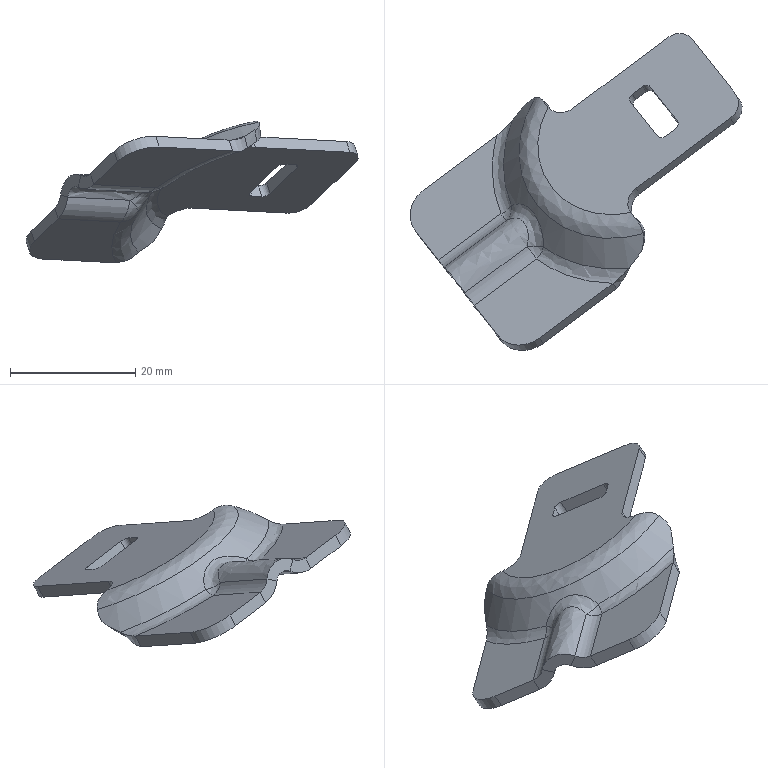Part | 1 solid | 62 faces | box 53.094 x 50.701 x 22.654 mm | volume 3030 mm3 | spline 54 | cylinder 4 | sphere 4 | commonest cylinder face diameters 6 x2 10 x2